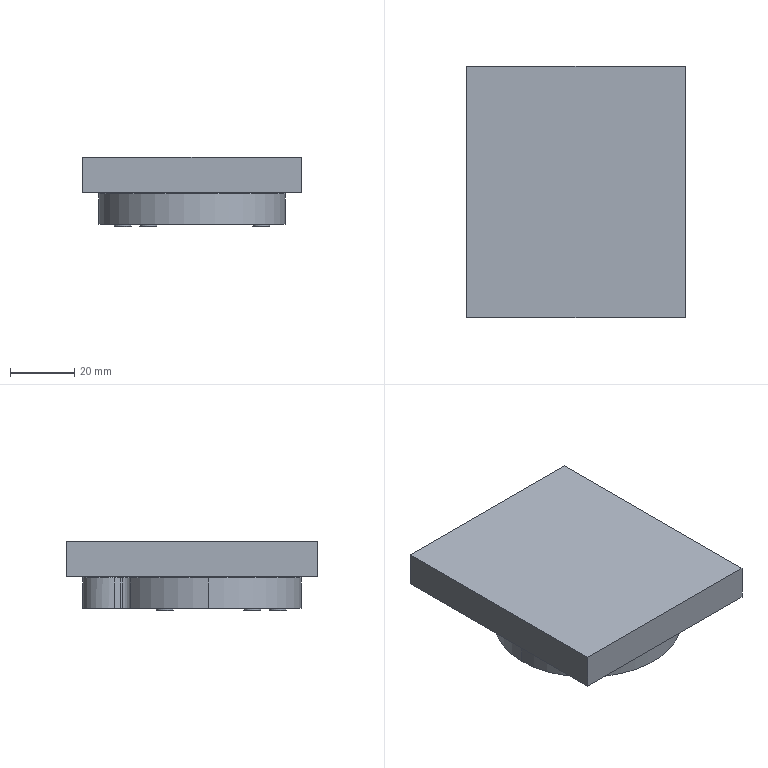NC program | NX | posted with a generic post | part box 68 x 78.27 x 21.8 mm
Lines 3557 to 4426 of 10371:
(ZLEVEL_PROFILE_1_1 , TOOL : D3R0.5)
N7076 T18 M6
N7078 G54
N7080 G17 G0 G90 X14.116 Y-30.582 S9500 M3
N7082 G43 Z30. H18
N7084 Z1.709
N7086 G94 G1 Z0.209 F1000.
N7088 X13.875 Y-30.164
N7090 G3 X13.615 Y-30.014 R0.3
N7092 G2 X10.299 Y-26.698 R3.316 F2500.
N7094 X13.615 Y-30.014 R-3.316
N7096 G1 X13.37 Y-30.004 Z0.208
N7098 X13.125 Y-29.979 Z0.207
N7100 X12.884 Y-29.932 Z0.206
N7102 X12.646 Y-29.873
N7104 X12.415 Y-29.789 Z0.205
N7106 X12.187 Y-29.696 Z0.204
N7108 X11.972 Y-29.577 Z0.203
N7110 X11.759 Y-29.455 Z0.202
N7112 X11.564 Y-29.304 Z0.201
N7114 X11.37 Y-29.152
N7116 X11.213 Y-28.988 Z0.2
N7118 X11.032 Y-28.795 Z0.199
N7120 X10.887 Y-28.595 Z0.198
N7122 X10.75 Y-28.391 Z0.197
N7124 X10.633 Y-28.173 Z0.196
N7126 X10.53 Y-27.95
N7128 X10.445 Y-27.718 Z0.195
N7130 X10.377 Y-27.481 Z0.194
N7132 X10.351 Y-27.359
N7134 X10.326 Y-27.237 Z0.193
N7136 X10.295 Y-26.99 Z0.192
N7138 X10.28 Y-26.741 Z0.191
N7140 X10.282 Y-26.616
N7142 X10.287 Y-26.492
N7144 X10.311 Y-26.243 Z0.19
N7146 X10.353 Y-25.997 Z0.189
N7148 X10.416 Y-25.756 Z0.188
N7150 X10.491 Y-25.518 Z0.187
N7152 X10.591 Y-25.289 Z0.186
N7154 X10.699 Y-25.064
N7156 X10.834 Y-24.854 Z0.185
N7158 X10.973 Y-24.646 Z0.184
N7160 X11.139 Y-24.459 Z0.183
N7162 X11.308 Y-24.275 Z0.182
N7164 X11.499 Y-24.113 Z0.181
N7166 X11.695 Y-23.958
N7168 X11.906 Y-23.823 Z0.18
N7170 X12.125 Y-23.702 Z0.179
N7172 X12.237 Y-23.646 Z0.178
N7174 X12.352 Y-23.597
N7176 X12.588 Y-23.512 Z0.177
N7178 X12.707 Y-23.474
N7180 X12.828 Y-23.441 Z0.176
N7182 X13.074 Y-23.392
N7184 X13.198 Y-23.375 Z0.175
N7186 X13.322 Y-23.358
N7188 X13.447 Y-23.351 Z0.174
N7190 X13.572 Y-23.347
N7192 X13.823 Y-23.351 Z0.173
N7194 X13.948 Y-23.36
N7196 X14.073 Y-23.377 Z0.172
N7198 X14.32 Y-23.419 Z0.171
N7200 X14.563 Y-23.48 Z0.17
N7202 X14.801 Y-23.562
N7204 X15.034 Y-23.654 Z0.169
N7206 X15.255 Y-23.773 Z0.168
N7208 X15.473 Y-23.897 Z0.167
N7210 X15.673 Y-24.049 Z0.166
N7212 X15.871 Y-24.204 Z0.165
N7214 X16.046 Y-24.384
N7216 X16.217 Y-24.568 Z0.164
N7218 X16.366 Y-24.771 Z0.163
N7220 X16.505 Y-24.98 Z0.162
N7222 X16.626 Y-25.201 Z0.161
N7224 X16.73 Y-25.43 Z0.16
N7226 X16.777 Y-25.547
N7228 X16.819 Y-25.665 Z0.159
N7230 X16.886 Y-25.908
N7232 X16.913 Y-26.031 Z0.158
N7234 X16.939 Y-26.154
N7236 X16.969 Y-26.404 Z0.157
N7238 X16.984 Y-26.656 Z0.156
N7240 X16.983 Y-26.781
N7242 X16.977 Y-26.907 Z0.155
N7244 X16.953 Y-27.158 Z0.154
N7246 X16.935 Y-27.283
N7248 X16.91 Y-27.406
N7250 X16.85 Y-27.638 Z0.153
N7252 X16.78 Y-27.867 Z0.152
N7254 X16.674 Y-28.11 Z0.151
N7256 X16.56 Y-28.349 Z0.15
N7258 X16.423 Y-28.561 Z0.149
N7260 X16.283 Y-28.771 Z0.148
N7262 X16.116 Y-28.96
N7264 X15.945 Y-29.147 Z0.147
N7266 X15.749 Y-29.313 Z0.146
N7268 X15.548 Y-29.472 Z0.145
N7270 X15.33 Y-29.609 Z0.144
N7272 X15.105 Y-29.733 Z0.143
N7274 X14.989 Y-29.79
N7276 X14.871 Y-29.838 Z0.142
N7278 X14.628 Y-29.925
N7280 X14.505 Y-29.964 Z0.141
N7282 X14.381 Y-29.996
N7284 X14.128 Y-30.043 Z0.14
N7286 X14. Y-30.061 Z0.139
N7288 X13.873 Y-30.076
N7290 X13.615 Y-30.084 Z0.138
N7292 X13.367 Y-30.079 Z0.137
N7294 X13.244 Y-30.066
N7296 X13.121 Y-30.05
N7298 X12.877 Y-30.007 Z0.136
N7300 X12.637 Y-29.944 Z0.135
N7302 X12.403 Y-29.863 Z0.134
N7304 X12.173 Y-29.769 Z0.133
N7306 X11.995 Y-29.674
N7308 X11.816 Y-29.577 Z0.132
N7310 X11.739 Y-29.529
N7312 X11.54 Y-29.381 Z0.131
N7314 X11.345 Y-29.227 Z0.13
N7316 X11.169 Y-29.052 Z0.129
N7318 X11.001 Y-28.869 Z0.128
N7320 X10.846 Y-28.668
N7322 X10.705 Y-28.456 Z0.127
N7324 X10.638 Y-28.348 Z0.126
N7326 X10.579 Y-28.235
N7328 X10.473 Y-28.004 Z0.125
N7330 X10.425 Y-27.886
N7332 X10.381 Y-27.767 Z0.124
N7334 X10.312 Y-27.522 Z0.123
N7336 X10.256 Y-27.273
N7338 X10.239 Y-27.147 Z0.122
N7340 X10.224 Y-27.021
N7342 X10.206 Y-26.767 Z0.121
N7344 Y-26.639 Z0.12
N7346 X10.212 Y-26.512
N7348 X10.234 Y-26.258 Z0.119
N7350 X10.276 Y-26.007 Z0.118
N7352 X10.338 Y-25.759 Z0.117
N7354 X10.413 Y-25.516
N7356 X10.514 Y-25.281 Z0.116
N7358 X10.623 Y-25.051 Z0.115
N7360 X10.758 Y-24.835 Z0.114
N7362 X10.9 Y-24.622 Z0.113
N7364 X11.066 Y-24.428 Z0.112
N7366 X11.239 Y-24.24
N7368 X11.43 Y-24.071 Z0.111
N7370 X11.631 Y-23.914 Z0.11
N7372 X11.815 Y-23.789 Z0.109
N7374 X12.007 Y-23.68 Z0.108
N7376 X12.068 Y-23.648
N7378 X12.181 Y-23.589
N7380 X12.298 Y-23.537 Z0.107
N7382 X12.539 Y-23.45
N7384 X12.661 Y-23.411 Z0.106
N7386 X12.783 Y-23.374
N7388 X12.909 Y-23.349 Z0.105
N7390 X13.034 Y-23.325
N7392 X13.288 Y-23.286 Z0.104
N7394 X13.415 Y-23.277
N7396 X13.544 Y-23.274 Z0.103
N7398 X13.8 Y-23.275 Z0.102
N7400 X13.928 Y-23.283
N7402 X14.055 Y-23.3
N7404 X14.308 Y-23.342 Z0.101
N7406 X14.557 Y-23.4 Z0.1
N7408 X14.8 Y-23.483 Z0.099
N7410 X15.04 Y-23.574 Z0.098
N7412 X15.266 Y-23.695 Z0.097
N7414 X15.49 Y-23.82 Z0.096
N7416 X15.697 Y-23.973
N7418 X15.899 Y-24.131 Z0.095
N7420 X16.081 Y-24.312 Z0.094
N7422 X16.256 Y-24.5 Z0.093
N7424 X16.412 Y-24.705 Z0.092
N7426 X16.554 Y-24.919 Z0.091
N7428 X16.622 Y-25.028
N7430 X16.682 Y-25.142
N7432 X16.788 Y-25.376 Z0.09
N7434 X16.838 Y-25.495 Z0.089
N7436 X16.882 Y-25.616
N7438 X16.951 Y-25.864 Z0.088
N7440 X16.98 Y-25.989
N7442 X17.009 Y-26.115 Z0.087
N7444 X17.026 Y-26.242
N7446 X17.04 Y-26.37 Z0.086
N7448 X17.055 Y-26.593
N7450 X17.056 Y-26.816 Z0.085
N7452 X17.052 Y-26.885
N7454 X17.03 Y-27.142 Z0.084
N7456 X16.988 Y-27.396 Z0.083
N7458 X16.925 Y-27.646 Z0.082
N7460 X16.85 Y-27.892 Z0.081
N7462 X16.748 Y-28.134 Z0.08
N7464 X16.634 Y-28.37
N7466 X16.496 Y-28.593 Z0.079
N7468 X16.347 Y-28.81 Z0.078
N7470 X16.177 Y-29.009 Z0.077
N7472 X15.997 Y-29.201 Z0.076
N7474 X15.798 Y-29.372 Z0.075
N7476 X15.59 Y-29.533 Z0.074
N7478 X15.48 Y-29.604
N7480 X15.369 Y-29.674 Z0.073
N7482 X15.138 Y-29.8
N7484 X15.018 Y-29.855 Z0.072
N7486 X14.899 Y-29.909
N7488 X14.651 Y-29.996 Z0.071
N7490 X14.398 Y-30.07 Z0.07
N7492 X14.139 Y-30.117 Z0.069
N7494 X13.878 Y-30.152 Z0.068
N7496 X13.615 Y-30.159 Z0.067
N7498 X13.373 Y-30.154
N7500 X13.253 Y-30.143 Z0.066
N7502 X13.133 Y-30.127
N7504 X12.895 Y-30.086 Z0.065
N7506 X12.66 Y-30.029 Z0.064
N7508 X12.431 Y-29.952
N7510 X12.205 Y-29.867 Z0.063
N7512 X11.989 Y-29.757 Z0.062
N7514 X11.777 Y-29.641 Z0.061
N7516 X11.563 Y-29.494 Z0.06
N7518 X11.358 Y-29.335
N7520 X11.167 Y-29.159 Z0.059
N7522 X10.989 Y-28.97 Z0.058
N7524 X10.903 Y-28.873 Z0.057
N7526 X10.824 Y-28.77
N7528 X10.678 Y-28.555 Z0.056
N7530 X10.609 Y-28.444
N7532 X10.543 Y-28.332 Z0.055
N7534 X10.432 Y-28.097
N7536 X10.332 Y-27.857 Z0.054
N7538 X10.293 Y-27.733 Z0.053
N7540 X10.257 Y-27.608
N7542 X10.196 Y-27.355 Z0.052
N7544 X10.172 Y-27.227
N7546 X10.157 Y-27.098 Z0.051
N7548 X10.136 Y-26.838 Z0.05
N7550 X10.134 Y-26.578
N7552 X10.154 Y-26.326 Z0.049
N7554 X10.184 Y-26.075 Z0.048
N7556 X10.247 Y-25.814 Z0.047
N7558 X10.318 Y-25.556 Z0.046
N7560 X10.417 Y-25.314 Z0.045
N7562 X10.523 Y-25.076 Z0.044
N7564 X10.657 Y-24.852
N7566 X10.799 Y-24.633 Z0.043
N7568 X10.962 Y-24.43 Z0.042
N7570 X11.138 Y-24.237 Z0.041
N7572 X11.229 Y-24.143
N7574 X11.327 Y-24.057 Z0.04
N7576 X11.531 Y-23.894 Z0.039
N7578 X11.636 Y-23.815
N7580 X11.744 Y-23.742
N7582 X11.972 Y-23.613 Z0.038
N7584 X12.088 Y-23.553 Z0.037
N7586 X12.205 Y-23.494
N7588 X12.327 Y-23.447
N7590 X12.449 Y-23.401 Z0.036
N7592 X12.698 Y-23.319 Z0.035
N7594 X12.824 Y-23.287
N7596 X12.953 Y-23.263 Z0.034
N7598 X13.211 Y-23.221
N7600 X13.341 Y-23.205 Z0.033
N7602 X13.472 Y-23.201
N7604 X13.734 Y-23.2 Z0.032
N7606 X13.996 Y-23.214 Z0.031
N7608 X14.254 Y-23.257 Z0.03
N7610 X14.511 Y-23.307 Z0.029
N7612 X14.76 Y-23.39
N7614 X15.007 Y-23.477 Z0.028
N7616 X15.241 Y-23.595 Z0.027
N7618 X15.472 Y-23.72 Z0.026
N7620 X15.687 Y-23.87 Z0.025
N7622 X15.895 Y-24.03 Z0.024
N7624 X16.088 Y-24.208 Z0.023
N7626 X16.267 Y-24.4
N7628 X16.355 Y-24.498 Z0.022
N7630 X16.435 Y-24.602
N7632 X16.581 Y-24.82 Z0.021
N7634 X16.652 Y-24.932
N7636 X16.718 Y-25.045 Z0.02
N7638 X16.83 Y-25.283 Z0.019
N7640 X16.931 Y-25.525 Z0.018
N7642 X16.971 Y-25.651
N7644 X17.006 Y-25.777
N7646 X17.069 Y-26.033 Z0.017
N7648 X17.093 Y-26.162 Z0.016
N7650 X17.107 Y-26.293
N7652 X17.129 Y-26.555 Z0.015
N7654 X17.132 Y-26.819 Z0.014
N7656 X17.112 Y-27.063 Z0.013
N7658 X17.086 Y-27.308
N7660 X17.027 Y-27.547 Z0.012
N7662 X16.968 Y-27.785 Z0.011
N7664 X16.879 Y-28.015 Z0.01
N7666 X16.782 Y-28.241 Z0.009
N7668 X16.669 Y-28.459
N7670 X16.538 Y-28.668 Z0.008
N7672 X16.468 Y-28.769 Z0.007
N7674 X16.396 Y-28.869
N7676 X16.317 Y-28.963
N7678 X16.236 Y-29.057 Z0.006
N7680 X16.067 Y-29.236 Z0.005
N7682 X15.978 Y-29.321
N7684 X15.884 Y-29.4
N7686 X15.689 Y-29.551 Z0.004
N7688 X15.488 Y-29.694 Z0.003
N7690 X15.271 Y-29.812 Z0.002
N7692 X15.054 Y-29.928 Z0.001
N7694 X14.804 Y-30.025
N7696 X14.59 Y-30.096 Z0.
N7698 X14.35 Y-30.155 Z-0.001
N7700 X14.108 Y-30.2 Z-0.002
N7702 X13.985 Y-30.216
N7704 X13.862 Y-30.229
N7706 X13.615 Y-30.236 Z-0.003
N7708 X13.357 Y-30.23 Z-0.004
N7710 X13.229 Y-30.217
N7712 X13.1 Y-30.201 Z-0.005
N7714 X12.846 Y-30.155 Z-0.006
N7716 X12.596 Y-30.091 Z-0.007
N7718 X12.352 Y-30.005
N7720 X12.112 Y-29.909 Z-0.008
N7722 X11.899 Y-29.801 Z-0.009
N7724 X11.778 Y-29.732
N7726 X11.66 Y-29.658 Z-0.01
N7728 X11.453 Y-29.504 Z-0.011
N7730 X11.249 Y-29.344
N7732 X11.066 Y-29.162 Z-0.012
N7734 X10.888 Y-28.973 Z-0.013
N7736 X10.731 Y-28.768 Z-0.014
N7738 X10.585 Y-28.554 Z-0.015
N7740 X10.456 Y-28.329
N7742 X10.345 Y-28.095 Z-0.016
N7744 X10.25 Y-27.853 Z-0.017
N7746 X10.175 Y-27.605 Z-0.018
N7748 X10.117 Y-27.352 Z-0.019
N7750 X10.077 Y-27.096 Z-0.02
N7752 X10.06 Y-26.837
N7754 X10.055 Y-26.578 Z-0.021
N7756 X10.078 Y-26.319 Z-0.022
N7758 X10.108 Y-26.061 Z-0.023
N7760 X10.165 Y-25.801 Z-0.024
N7762 X10.202 Y-25.673
N7764 X10.24 Y-25.545
N7766 X10.287 Y-25.42 Z-0.025
N7768 X10.335 Y-25.296
N7770 X10.448 Y-25.055 Z-0.026
N7772 X10.51 Y-24.936 Z-0.027
N7774 X10.579 Y-24.822
N7776 X10.727 Y-24.6 Z-0.028
N7778 X10.804 Y-24.491
N7780 X10.891 Y-24.39 Z-0.029
N7782 X11.07 Y-24.192 Z-0.03
N7784 X11.163 Y-24.096
N7786 X11.264 Y-24.009
N7788 X11.471 Y-23.84 Z-0.031
N7790 X11.617 Y-23.736 Z-0.032
N7792 X11.768 Y-23.638
N7794 X11.92 Y-23.551 Z-0.033
N7796 X12.159 Y-23.431 Z-0.034
N7798 X12.282 Y-23.38
N7800 X12.407 Y-23.332 Z-0.035
N7802 X12.662 Y-23.249
N7804 X12.791 Y-23.214 Z-0.036
N7806 X12.922 Y-23.188
N7808 X13.186 Y-23.145 Z-0.037
N7810 X13.319 Y-23.127 Z-0.038
N7812 X13.453 Y-23.122
N7814 X13.72 Y-23.119 Z-0.039
N7816 X13.854 Y-23.122
N7818 X13.988 Y-23.135 Z-0.04
N7820 X14.253 Y-23.173
N7822 X14.384 Y-23.199 Z-0.041
N7824 X14.515 Y-23.228
N7826 X14.772 Y-23.306 Z-0.042
N7828 X15.023 Y-23.399 Z-0.043
N7830 X15.145 Y-23.455
N7832 X15.265 Y-23.515 Z-0.044
N7834 X15.499 Y-23.646 Z-0.045
N7836 X15.614 Y-23.716
N7838 X15.722 Y-23.795 Z-0.046
N7840 X15.934 Y-23.96
N7842 X16.037 Y-24.046 Z-0.047
N7844 X16.132 Y-24.141
N7846 X16.317 Y-24.336 Z-0.048
N7848 X16.406 Y-24.437
N7850 X16.488 Y-24.543 Z-0.049
N7852 X16.641 Y-24.764 Z-0.05
N7854 X16.71 Y-24.879
N7856 X16.779 Y-24.994 Z-0.051
N7858 X16.897 Y-25.236
N7860 X17. Y-25.485 Z-0.052
N7862 X17.042 Y-25.612 Z-0.053
N7864 X17.079 Y-25.742
N7866 X17.143 Y-26.003 Z-0.054
N7868 X17.169 Y-26.135
N7870 X17.185 Y-26.269 Z-0.055
N7872 X17.213 Y-26.626 Z-0.056
N7874 X17.215 Y-26.716
N7876 X17.211 Y-26.806 Z-0.057
N7878 X17.193 Y-27.075
N7880 X17.179 Y-27.209 Z-0.058
N7882 X17.158 Y-27.342
N7884 X17.099 Y-27.605 Z-0.059
N7886 X17.025 Y-27.864 Z-0.06
N7888 X16.926 Y-28.115 Z-0.061
N7890 X16.814 Y-28.36 Z-0.062
N7892 X16.749 Y-28.478
N7894 X16.679 Y-28.594
N7896 X16.53 Y-28.818 Z-0.063
N7898 X16.452 Y-28.928 Z-0.064
N7900 X16.364 Y-29.031
N7902 X16.182 Y-29.23 Z-0.065
N7904 X16.088 Y-29.327
N7906 X15.987 Y-29.417 Z-0.066
N7908 X15.777 Y-29.587 Z-0.067
N7910 X15.668 Y-29.666
N7912 X15.557 Y-29.743 Z-0.068
N7914 X15.323 Y-29.878
N7916 X15.082 Y-30.001 Z-0.069
N7918 X14.957 Y-30.05 Z-0.07
N7920 X14.831 Y-30.1
N7922 X14.634 Y-30.162 Z-0.071
N7924 X14.435 Y-30.22
N7926 X14.028 Y-30.29 Z-0.073
N7928 X13.822 Y-30.309
N7930 X13.615 Y-30.315 Z-0.074
N7932 X13.387 Y-30.309 Z-0.075
N7934 X13.159 Y-30.288
N7936 X12.709 Y-30.209 Z-0.077
N7938 X12.275 Y-30.064 Z-0.078
N7940 X12.066 Y-29.972 Z-0.079
N7942 X11.861 Y-29.871 Z-0.08
N7944 X11.643 Y-29.741
N7946 X11.435 Y-29.597 Z-0.081
N7948 X11.239 Y-29.437 Z-0.082
N7950 X11.051 Y-29.267 Z-0.083
N7952 X10.882 Y-29.078 Z-0.084
N7954 X10.715 Y-28.888
N7956 X10.573 Y-28.678 Z-0.085
N7958 X10.436 Y-28.464 Z-0.086
N7960 X10.325 Y-28.236 Z-0.087
N7962 X10.221 Y-28.005
N7964 X10.142 Y-27.764 Z-0.088
N7966 X10.073 Y-27.52 Z-0.089
N7968 X10.047 Y-27.396
N7970 X10.022 Y-27.271 Z-0.09
N7972 X10.005 Y-27.146
N7974 X9.991 Y-27.019 Z-0.091
N7976 X9.976 Y-26.766
N7978 X9.979 Y-26.512 Z-0.092
N7980 X10. Y-26.259 Z-0.093
N7982 X10.036 Y-26.008 Z-0.094
N7984 X10.094 Y-25.76
N7986 X10.163 Y-25.515 Z-0.095
N7988 X10.256 Y-25.279 Z-0.096
N7990 X10.361 Y-25.047 Z-0.097
N7992 X10.484 Y-24.824 Z-0.098
N7994 X10.622 Y-24.61
N7996 X10.775 Y-24.407 Z-0.099
N7998 X10.94 Y-24.213 Z-0.1
N8000 X11.12 Y-24.032 Z-0.101
N8002 X11.31 Y-23.863
N8004 X11.513 Y-23.709 Z-0.102
N8006 X11.725 Y-23.568 Z-0.103
N8008 X11.948 Y-23.443 Z-0.104
N8010 X12.178 Y-23.334 Z-0.105
N8012 X12.416 Y-23.241
N8014 X12.659 Y-23.166 Z-0.106
N8016 X12.908 Y-23.106 Z-0.107
N8018 X13.16 Y-23.065 Z-0.108
N8020 X13.414 Y-23.041 Z-0.109
N8022 X13.669 Y-23.035
N8024 X13.925 Y-23.05 Z-0.11
N8026 X14.179 Y-23.077 Z-0.111
N8028 X14.43 Y-23.124 Z-0.112
N8030 X14.677 Y-23.189
N8032 X14.92 Y-23.27 Z-0.113
N8034 X15.156 Y-23.369 Z-0.114
N8036 X15.385 Y-23.484 Z-0.115
N8038 X15.605 Y-23.615 Z-0.116
N8040 X15.816 Y-23.76
N8042 X16.016 Y-23.92 Z-0.117
N8044 X16.204 Y-24.094 Z-0.118
N8046 X16.38 Y-24.28 Z-0.119
N8048 X16.543 Y-24.479 Z-0.12
N8050 X16.691 Y-24.688
N8052 X16.825 Y-24.907 Z-0.121
N8054 X16.943 Y-25.135 Z-0.122
N8056 X17.044 Y-25.371 Z-0.123
N8058 X17.129 Y-25.613
N8060 X17.197 Y-25.861 Z-0.124
N8062 X17.248 Y-26.113 Z-0.125
N8064 X17.281 Y-26.368 Z-0.126
N8066 X17.296 Y-26.624 Z-0.127
N8068 X17.292 Y-26.89
N8070 X17.269 Y-27.155 Z-0.128
N8072 X17.228 Y-27.419 Z-0.129
N8074 X17.167 Y-27.678 Z-0.13
N8076 X17.088 Y-27.932 Z-0.131
N8078 X16.99 Y-28.18 Z-0.132
N8080 X16.875 Y-28.421
N8082 X16.743 Y-28.652 Z-0.133
N8084 X16.594 Y-28.873 Z-0.134
N8086 X16.43 Y-29.083 Z-0.135
N8088 X16.251 Y-29.281 Z-0.136
N8090 X16.058 Y-29.466
N8092 X15.852 Y-29.636 Z-0.137
N8094 X15.634 Y-29.79 Z-0.138
N8096 X15.406 Y-29.929 Z-0.139
N8098 X15.169 Y-30.051 Z-0.14
N8100 X14.922 Y-30.155 Z-0.141
N8102 X14.67 Y-30.241
N8104 X14.508 Y-30.286 Z-0.142
N8106 X14.345 Y-30.323
N8108 X14.247 Y-30.342 Z-0.143
N8110 X14.148 Y-30.358
N8112 X13.883 Y-30.388 Z-0.144
N8114 X13.615 Y-30.399 Z-0.145
N8116 X13.48 Y-30.397
N8118 X13.346 Y-30.39 Z-0.146
N8120 X13.211 Y-30.378
N8122 X13.077 Y-30.361
N8124 X12.944 Y-30.34 Z-0.147
N8126 X12.811 Y-30.313
N8128 X12.68 Y-30.282 Z-0.148
N8130 X12.55 Y-30.246
N8132 X12.421 Y-30.205
N8134 X12.294 Y-30.16 Z-0.149
N8136 X12.168 Y-30.11
N8138 X12.045 Y-30.055 Z-0.15
N8140 X11.923 Y-29.996
N8142 X11.804 Y-29.933
N8144 X11.687 Y-29.865 Z-0.151
N8146 X11.572 Y-29.793
N8148 X11.461 Y-29.717 Z-0.152
N8150 X11.352 Y-29.636
N8152 X11.246 Y-29.552
N8154 X11.143 Y-29.464 Z-0.153
N8156 X11.044 Y-29.373
N8158 X10.947 Y-29.278 Z-0.154
N8160 X10.855 Y-29.179
N8162 X10.766 Y-29.077
N8164 X10.681 Y-28.972 Z-0.155
N8166 X10.599 Y-28.864
N8168 X10.522 Y-28.753 Z-0.156
N8170 X10.428 Y-28.605
N8172 X10.306 Y-28.386 Z-0.157
N8174 X10.199 Y-28.159 Z-0.158
N8176 X10.147 Y-28.034
N8178 X10.1 Y-27.907 Z-0.159
N8180 X10.058 Y-27.778
N8182 X10.021 Y-27.648
N8184 X9.988 Y-27.516 Z-0.16
N8186 X9.96 Y-27.383
N8188 X9.937 Y-27.25 Z-0.161
N8190 X9.919 Y-27.116
N8192 X9.905 Y-26.962
N8194 X9.896 Y-26.808 Z-0.162
N8196 X9.894 Y-26.691
N8198 X9.896 Y-26.574 Z-0.163
N8200 X9.902 Y-26.439
N8202 X9.914 Y-26.304
N8204 X9.93 Y-26.169 Z-0.164
N8206 X9.952 Y-26.035
N8208 X9.978 Y-25.902 Z-0.165
N8210 X10.009 Y-25.77
N8212 X10.045 Y-25.639
N8214 X10.085 Y-25.509 Z-0.166
N8216 X10.176 Y-25.266 Z-0.167
N8218 X10.283 Y-25.029
N8220 X10.407 Y-24.8 Z-0.168
N8222 X10.547 Y-24.581 Z-0.169
N8224 X10.701 Y-24.372 Z-0.17
N8226 X10.87 Y-24.174 Z-0.171
N8228 X11.052 Y-23.988
N8230 X11.247 Y-23.815 Z-0.172
N8232 X11.453 Y-23.656 Z-0.173
N8234 X11.67 Y-23.512 Z-0.174
N8236 X11.896 Y-23.384 Z-0.175
N8238 X12.131 Y-23.271
N8240 X12.374 Y-23.176 Z-0.176
N8242 X12.622 Y-23.097 Z-0.177
N8244 X12.876 Y-23.036 Z-0.178
N8246 X13.133 Y-22.992
N8248 X13.392 Y-22.967 Z-0.179
N8250 X13.653 Y-22.96 Z-0.18
N8252 X13.913 Y-22.971 Z-0.181
N8254 X14.173 Y-23. Z-0.182
N8256 X14.316 Y-23.024
N8258 X14.458 Y-23.054
N8260 X14.57 Y-23.081 Z-0.183
N8262 X14.682 Y-23.112
N8264 X14.93 Y-23.195 Z-0.184
N8266 X15.171 Y-23.295 Z-0.185
N8268 X15.405 Y-23.411 Z-0.186
N8270 X15.63 Y-23.543
N8272 X15.846 Y-23.691 Z-0.187
N8274 X16.051 Y-23.853 Z-0.188
N8276 X16.244 Y-24.03 Z-0.189
N8278 X16.424 Y-24.219
N8280 X16.591 Y-24.421 Z-0.19
N8282 X16.743 Y-24.634 Z-0.191
N8284 X16.88 Y-24.857 Z-0.192
N8286 X17.001 Y-25.088 Z-0.193
N8288 X17.106 Y-25.328
N8290 X17.193 Y-25.575 Z-0.194
N8292 X17.264 Y-25.827 Z-0.195
N8294 X17.316 Y-26.084 Z-0.196
N8296 X17.351 Y-26.344 Z-0.197
N8298 X17.367 Y-26.605
N8300 X17.368 Y-26.652
N8302 Y-26.7 Z-0.198
N8304 X17.363 Y-26.914
N8306 X17.345 Y-27.129 Z-0.199
N8308 X17.306 Y-27.388 Z-0.2
N8310 X17.25 Y-27.644
N8312 X17.176 Y-27.896 Z-0.201
N8314 X17.084 Y-28.141 Z-0.202
N8316 X16.976 Y-28.38 Z-0.203
N8318 X16.851 Y-28.611 Z-0.204
N8320 X16.769 Y-28.744
N8322 X16.682 Y-28.873 Z-0.205
N8324 X16.619 Y-28.959
N8326 X16.554 Y-29.044
N8328 X16.384 Y-29.244 Z-0.206
N8330 X16.2 Y-29.432 Z-0.207
N8332 X16.003 Y-29.606 Z-0.208
N8334 X15.795 Y-29.766
N8336 X15.576 Y-29.912 Z-0.209
N8338 X15.347 Y-30.041 Z-0.21
N8340 X15.11 Y-30.155 Z-0.211
N8342 X14.865 Y-30.252 Z-0.212
N8344 X14.615 Y-30.331
N8346 X14.359 Y-30.393 Z-0.213
N8348 X14.175 Y-30.426 Z-0.214
N8350 X13.989 Y-30.449
N8352 X13.802 Y-30.464 Z-0.215
N8354 X13.615 Y-30.469
N8356 X13.372 Y-30.462 Z-0.216
N8358 X13.13 Y-30.44 Z-0.217
N8360 X12.89 Y-30.401 Z-0.218
N8362 X12.652 Y-30.348
N8364 X12.419 Y-30.279 Z-0.219
N8366 X12.19 Y-30.195 Z-0.22
N8368 X11.967 Y-30.097
N8370 X11.751 Y-29.984 Z-0.221
N8372 X11.543 Y-29.858 Z-0.222
N8374 X11.343 Y-29.719 Z-0.223
N8376 X11.153 Y-29.567
N8378 X10.973 Y-29.403 Z-0.224
N8380 X10.803 Y-29.227 Z-0.225
N8382 X10.645 Y-29.041
N8384 X10.5 Y-28.846 Z-0.226
N8386 X10.346 Y-28.605 Z-0.227
N8388 X10.24 Y-28.412 Z-0.228
N8390 X10.145 Y-28.213
N8392 X10.055 Y-27.99 Z-0.229
N8394 X9.979 Y-27.761 Z-0.23
N8396 X9.918 Y-27.527
N8398 X9.872 Y-27.29 Z-0.231
N8400 X9.841 Y-27.051 Z-0.232
N8402 X9.826 Y-26.81 Z-0.233
N8404 X9.824 Y-26.761
N8406 Y-26.712
N8408 X9.828 Y-26.495 Z-0.234
N8410 X9.846 Y-26.278
N8412 X9.884 Y-26.014 Z-0.235
N8414 X9.94 Y-25.753 Z-0.236
N8416 X10.015 Y-25.497 Z-0.237
N8418 X10.107 Y-25.247
N8420 X10.217 Y-25.004 Z-0.238
N8422 X10.344 Y-24.769 Z-0.239
N8424 X10.486 Y-24.544 Z-0.24
N8426 X10.645 Y-24.329 Z-0.241
N8428 X10.818 Y-24.125
N8430 X11.005 Y-23.935 Z-0.242
N8432 X11.205 Y-23.758 Z-0.243
N8434 X11.417 Y-23.595 Z-0.244
N8436 X11.64 Y-23.448
N8438 X11.873 Y-23.316 Z-0.245
N8440 X12.114 Y-23.202 Z-0.246
N8442 X12.363 Y-23.104 Z-0.247
N8444 X12.619 Y-23.024 Z-0.248
N8446 X12.879 Y-22.963
N8448 X13.143 Y-22.92 Z-0.249
N8450 X13.41 Y-22.895 Z-0.25
N8452 X13.677 Y-22.889 Z-0.251
N8454 X13.945 Y-22.903 Z-0.252
N8456 X14.211 Y-22.934
N8458 X14.474 Y-22.985 Z-0.253
N8460 X14.601 Y-23.016 Z-0.254
N8462 X14.728 Y-23.052
N8464 X14.847 Y-23.09
N8466 X14.964 Y-23.132 Z-0.255
N8468 X15.2 Y-23.23
N8470 X15.43 Y-23.344 Z-0.256
N8472 X15.651 Y-23.473 Z-0.257
N8474 X15.864 Y-23.616 Z-0.258
N8476 X16.066 Y-23.774
N8478 X16.257 Y-23.944 Z-0.259
N8480 X16.437 Y-24.128 Z-0.26
N8482 X16.603 Y-24.322 Z-0.261
N8484 X16.757 Y-24.528
N8486 X16.896 Y-24.744 Z-0.262
N8488 X17.02 Y-24.968 Z-0.263
N8490 X17.129 Y-25.2 Z-0.264
N8492 X17.223 Y-25.44 Z-0.265
N8494 X17.3 Y-25.685
N8496 X17.36 Y-25.934 Z-0.266
N8498 X17.403 Y-26.187 Z-0.267
N8500 X17.43 Y-26.443 Z-0.268
N8502 X17.439 Y-26.7
N8504 X17.432 Y-26.935 Z-0.269
N8506 X17.411 Y-27.17 Z-0.27
N8508 X17.375 Y-27.403
N8510 X17.325 Y-27.634 Z-0.271
N8512 X17.261 Y-27.861 Z-0.272
N8514 X17.184 Y-28.083 Z-0.273
N8516 X17.092 Y-28.301
N8518 X16.987 Y-28.512 Z-0.274
N8520 X16.883 Y-28.696 Z-0.275
N8522 X16.74 Y-28.914
N8524 X16.582 Y-29.122 Z-0.276
N8526 X16.411 Y-29.319 Z-0.277
N8528 X16.226 Y-29.504 Z-0.278
N8530 X16.03 Y-29.676
N8532 X15.822 Y-29.834 Z-0.279
N8534 X15.604 Y-29.977 Z-0.28
N8536 X15.376 Y-30.106 Z-0.281
N8538 X15.141 Y-30.219
N8540 X14.898 Y-30.315 Z-0.282
N8542 X14.649 Y-30.395 Z-0.283
N8544 X14.395 Y-30.457 Z-0.284
N8546 X14.137 Y-30.503 Z-0.285
N8548 X13.877 Y-30.53
N8550 X13.615 Y-30.54 Z-0.286
N8552 X13.365 Y-30.533 Z-0.287
N8554 X13.116 Y-30.509 Z-0.288
N8556 X12.868 Y-30.469
N8558 X12.624 Y-30.413 Z-0.289
N8560 X12.384 Y-30.342 Z-0.29
N8562 X12.149 Y-30.255
N8564 X11.92 Y-30.152 Z-0.291
N8566 X11.698 Y-30.035 Z-0.292
N8568 X11.484 Y-29.904 Z-0.293
N8570 X11.28 Y-29.759
N8572 X11.085 Y-29.601 Z-0.294
N8574 X10.9 Y-29.431 Z-0.295
N8576 X10.728 Y-29.249 Z-0.296
N8578 X10.567 Y-29.056
N8580 X10.489 Y-28.952 Z-0.297
N8582 X10.414 Y-28.846
N8584 X10.348 Y-28.744
N8586 X10.285 Y-28.641 Z-0.298
N8588 X10.164 Y-28.419
N8590 X10.058 Y-28.189 Z-0.299
N8592 X9.967 Y-27.953 Z-0.3
N8594 X9.892 Y-27.712 Z-0.301
N8596 X9.833 Y-27.466
N8598 X9.79 Y-27.217 Z-0.302
N8600 X9.763 Y-26.965 Z-0.303
N8602 X9.753 Y-26.713 Z-0.304
N8604 X9.754 Y-26.574
N8606 X9.761 Y-26.435
N8608 X9.773 Y-26.296 Z-0.305
N8610 X9.789 Y-26.158
N8612 X9.811 Y-26.021 Z-0.306
N8614 X9.837 Y-25.884
N8616 X9.868 Y-25.749
N8618 X9.904 Y-25.614 Z-0.307
N8620 X9.945 Y-25.482
N8622 X9.991 Y-25.35 Z-0.308
N8624 X10.042 Y-25.221
N8626 X10.097 Y-25.093
N8628 X10.156 Y-24.967 Z-0.309
N8630 X10.22 Y-24.844
N8632 X10.289 Y-24.722 Z-0.31
N8634 X10.362 Y-24.604
N8636 X10.439 Y-24.488
N8638 X10.52 Y-24.375 Z-0.311
N8640 X10.605 Y-24.265
N8642 X10.694 Y-24.158 Z-0.312
N8644 X10.787 Y-24.054
N8646 X10.884 Y-23.954 Z-0.313
N8648 X10.984 Y-23.857
N8650 X11.088 Y-23.764
N8652 X11.195 Y-23.675 Z-0.314
N8654 X11.305 Y-23.589
N8656 X11.418 Y-23.508 Z-0.315
N8658 X11.534 Y-23.431
N8660 X11.653 Y-23.358
N8662 X11.774 Y-23.289 Z-0.316
N8664 X11.897 Y-23.225
N8666 X12.023 Y-23.165 Z-0.317
N8668 X12.151 Y-23.109
N8670 X12.281 Y-23.059
N8672 X12.413 Y-23.013 Z-0.318
N8674 X12.546 Y-22.971
N8676 X12.681 Y-22.935 Z-0.319
N8678 X12.817 Y-22.904
N8680 X12.954 Y-22.877
N8682 X13.091 Y-22.855 Z-0.32
N8684 X13.23 Y-22.839
N8686 X13.369 Y-22.827 Z-0.321
N8688 X13.508 Y-22.82
N8690 X13.648 Y-22.818
N8692 X13.788 Y-22.822 Z-0.322
N8694 X13.927 Y-22.83
N8696 X14.066 Y-22.844 Z-0.323
N8698 X14.204 Y-22.862
N8700 X14.342 Y-22.885
N8702 X14.479 Y-22.914 Z-0.324
N8704 X14.615 Y-22.947
N8706 X14.749 Y-22.985 Z-0.325
N8708 X14.849 Y-23.017
N8710 X14.949 Y-23.051
N8712 X15.107 Y-23.113 Z-0.326
N8714 X15.262 Y-23.181
N8716 X15.508 Y-23.306 Z-0.327
N8718 X15.743 Y-23.448 Z-0.328
N8720 X15.968 Y-23.606 Z-0.329
N8722 X16.182 Y-23.78
N8724 X16.383 Y-23.968 Z-0.33
N8726 X16.569 Y-24.171 Z-0.331
N8728 X16.741 Y-24.386 Z-0.332
N8730 X16.898 Y-24.612 Z-0.333
N8732 X17.038 Y-24.85
N8734 X17.161 Y-25.096 Z-0.334
N8736 X17.266 Y-25.351 Z-0.335
N8738 X17.353 Y-25.613 Z-0.336
N8740 X17.421 Y-25.88 Z-0.337
N8742 X17.47 Y-26.152
N8744 X17.5 Y-26.426 Z-0.338
N8746 X17.51 Y-26.702 Z-0.339
N8748 X17.503 Y-26.936 Z-0.34
N8750 X17.482 Y-27.17
N8752 X17.447 Y-27.403 Z-0.341
N8754 X17.399 Y-27.632 Z-0.342
N8756 X17.336 Y-27.859
N8758 X17.26 Y-28.081 Z-0.343
N8760 X17.171 Y-28.298 Z-0.344
N8762 X17.068 Y-28.51 Z-0.345
N8764 X16.974 Y-28.681
N8766 X16.87 Y-28.848 Z-0.346
N8768 X16.849 Y-28.88
N8770 X16.826 Y-28.913
N8772 X16.666 Y-29.13 Z-0.347
N8774 X16.492 Y-29.335
N8776 X16.304 Y-29.528 Z-0.348
N8778 X16.102 Y-29.707 Z-0.349
N8780 X15.889 Y-29.873 Z-0.35
N8782 X15.665 Y-30.023 Z-0.351
N8784 X15.431 Y-30.157
N8786 X15.189 Y-30.275 Z-0.352
N8788 X14.938 Y-30.376 Z-0.353
N8790 X14.682 Y-30.459 Z-0.354
N8792 X14.42 Y-30.524
N8794 X14.154 Y-30.572 Z-0.355
N8796 X13.885 Y-30.601 Z-0.356
N8798 X13.615 Y-30.611 Z-0.357
N8800 X13.342 Y-30.602 Z-0.358
N8802 X13.069 Y-30.574
N8804 X12.799 Y-30.527 Z-0.359
N8806 X12.533 Y-30.462 Z-0.36
N8808 X12.272 Y-30.378 Z-0.361